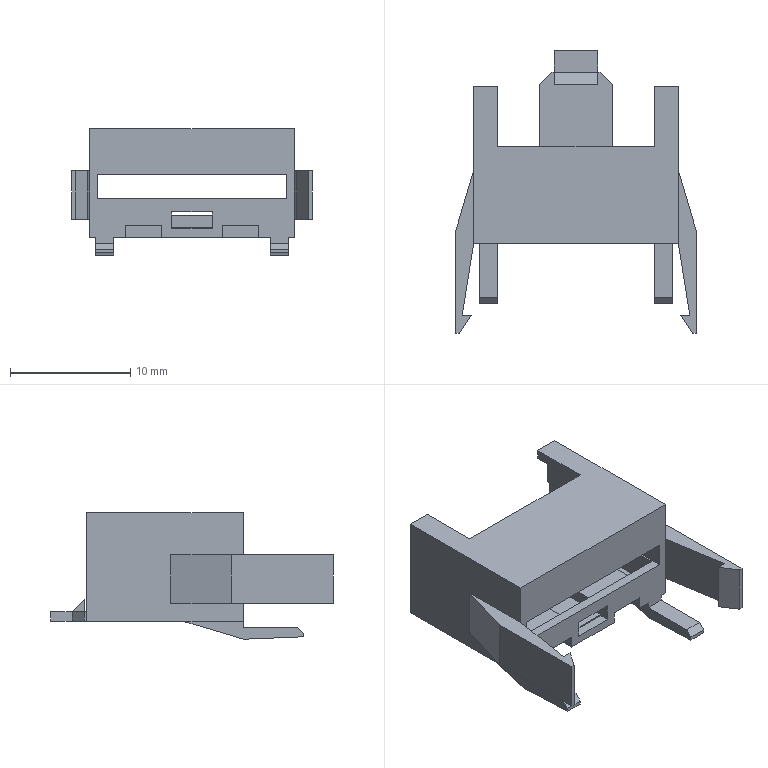Part | STEP file | LIANJIEQI2_14_1 | 1 solid | 115 faces | box 20 x 23.5 x 10.5 mm | volume 729.279 mm3 | plane 115